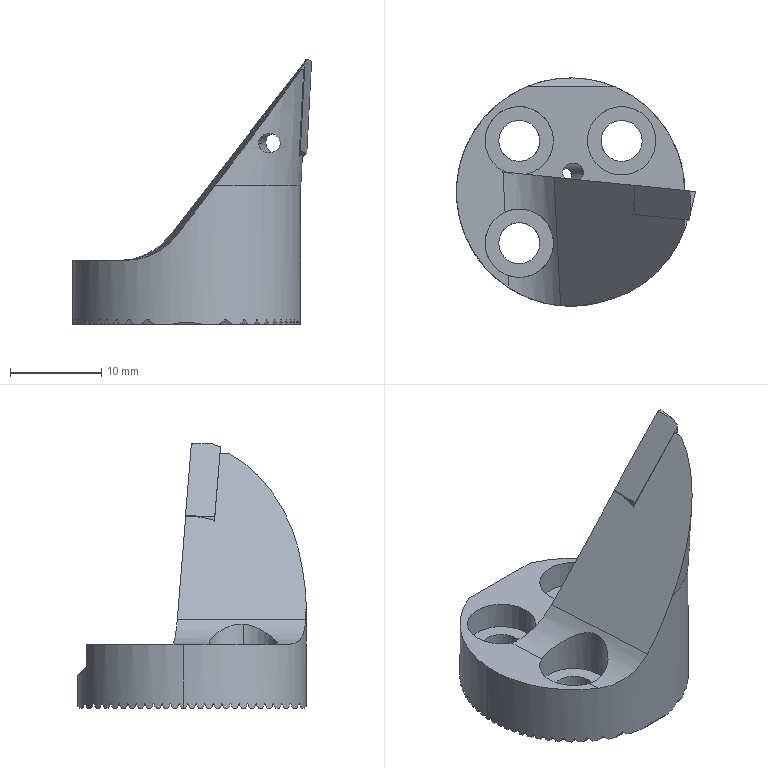CAM job | Mastercam | 3-axis milling, 5-axis milling, drilling
Tools:
tool_number,name,type,diameter_mm,corner_radius_mm,flutes,flute_length_mm,overall_length_mm,shoulder_length_mm,holder_diameter_mm,length_offset,diameter_offset,default_rpm,default_feed_mm_min,default_plunge_mm_min,coolant
1,6 Flat End Mill,end mill,6,0,4,23,23,23,31.877,1,1,1667,200.04,600,COOL_OFF
2,2 Drill,drill,2,0,2,30,30,30,31.877,2,2,3000,360,600,COOL_OFF
4,12 Flat End Mill Rough,end mill,12,0,4,25,25,25,42.012,4,4,833,99.96,600,COOL_OFF
5,3 Flat End Mill Rough,end mill,3,0,4,20,20,20,27.495,5,5,3334,400.08,600,COOL_OFF
6,3 Flat End Mill Rough,end mill,3,0,4,20,20,20,31.877,6,6,3333,399.96,600,COOL_OFF
7,3 Flat End Mill Finish,end mill,3,0,4,20,20,20,31.877,7,7,3333,399.96,600,COOL_OFF
8,2x7deg Chamfer Mill,chamfer mill,6,0,4,12,20,20,31.877,8,8,4167,500.04,600,COOL_OFF
9,12 Flat End Mill Finish,end mill,12,0,4,25,25,25,42.012,9,9,833,99.96,600,COOL_OFF
10,30 Bull Nose Mill,bull end mill,30,0.8,4,30,30,30,50,10,10,400,48,600,COOL_OFF
11,2.5 Flat End Mill,end mill,2.5,0,4,20,20,20,31.877,11,11,4000,480,600,COOL_OFF
12,5 Spot Drill,drill,5,0,2,25,25,25,31.877,12,12,1200,144,600,COOL_OFF
13,2.1 Drill,drill,2.1,0,2,20,20,20,31.877,13,13,2857,342.84,600,COOL_OFF
14,1.95 Thread Mill,thread mill,1.95,0,4,1.35,15,15,31.877,14,14,3077,369.24,600,COOL_OFF
15,2.5 Ball Mill,ball end mill,2.5,1.25,4,3,20,3,31.877,15,15,4800,576,600,COOL_OFF
Operations:
seq,operation,operation_type,tool_number,tool_name,tool_diameter_mm,spindle_rpm,feed_mm_min,plunge_mm_min,retract_mm_min,cycle_time_s,wcs,posted,nc_file
1,2D High Speed (2D Dynamic Mill) - [WCS: Top] - [Tplane: Ins],HighSpeed2D,4,12 Flat End Mill Rough,12,3500,2500,2000,1200,75.295,Top,yes,.nc
2,2D High Speed (2D Dynamic Mill) - [WCS: Top] - [Tplane: Ins-1],HighSpeed2D,4,12 Flat End Mill Rough,12,3500,2500,2000,1200,66.868,Top,yes,.nc
3,Contour (2D) - [WCS: Top] - [Tplane: Out],Contour,1,6 Flat End Mill,6,3500,400,2000,1200,19.183,Top,yes,.nc
4,Peck Drill - [WCS: Top] - [Tplane: Out],Drill,2,2 Drill,2,150,10,600,1200,57.614,Top,yes,.nc
5,2D High Speed (2D Dynamic Mill) - [WCS: Top] - [Tplane: Ins],HighSpeed2D,4,12 Flat End Mill Rough,12,3500,2500,2000,1200,18.885,Top,yes,.nc
6,Contour (2D) - [WCS: Top] - [Tplane: Ins],Contour,4,12 Flat End Mill Rough,12,3500,1000,2000,1200,6.261,Top,yes,.nc
7,Contour (Ramp) - [WCS: Top] - [Tplane: 0d],Contour,4,12 Flat End Mill Rough,12,3500,1500,2000,1200,2.576,Top,yes,.nc
8,Contour (Ramp) - [WCS: Top] - [Tplane: 45d],Contour,4,12 Flat End Mill Rough,12,3500,1500,2000,1200,2.436,Top,yes,.nc
9,Contour (2D) - [WCS: Top] - [Tplane: Ins],Contour,6,3 Flat End Mill Rough,3,4500,400,2000,1200,180.495,Top,yes,.nc
10,Contour (2D) - [WCS: Top] - [Tplane: Ins],Contour,7,3 Flat End Mill Finish,3,4500,400,2000,1200,10.995,Top,yes,.nc
11,Contour (2D) - [WCS: Top] - [Tplane: Ins],Contour,7,3 Flat End Mill Finish,3,4500,400,2000,1200,10.995,Top,yes,.nc
12,Contour (2D chamfer) - [WCS: Top] - [Tplane: Ins],Contour,8,2x7deg Chamfer Mill,6,3500,400,2000,1200,9.64,Top,yes,.nc
13,Contour (2D) - [WCS: Top] - [Tplane: Ins-1],Contour,9,12 Flat End Mill Finish,12,3500,600,2000,1200,5.675,Top,yes,.nc
14,Contour (2D) - [WCS: Top] - [Tplane: Ins],Contour,9,12 Flat End Mill Finish,12,3500,600,2000,1200,4.903,Top,yes,.nc
15,Contour (2D) - [WCS: Top] - [Tplane: 0d],Contour,9,12 Flat End Mill Finish,12,3500,600,2000,1200,3.055,Top,yes,.nc
16,Contour (2D) - [WCS: Top] - [Tplane: 45d],Contour,9,12 Flat End Mill Finish,12,3500,600,2000,1200,2.916,Top,yes,.nc
17,Contour (2D) - [WCS: Top] - [Tplane: Ins],Contour,10,30 Bull Nose Mill,30,3000,400,2000,1200,10.103,Top,yes,.nc
18,Drill/Counterbore - [WCS: Top] - [Tplane: Ins],Drill,12,5 Spot Drill,5,2000,100,600,1200,1.919,Top,yes,.nc
19,Peck Drill - [WCS: Top] - [Tplane: Ins],Drill,13,2.1 Drill,2.1,2500,40,600,1200,14.202,Top,yes,.nc
20,Peck Drill - [WCS: Top] - [Tplane: Plane],Drill,11,2.5 Flat End Mill,2.5,4000,40,600,1200,6.243,Top,yes,.nc
21,Thread Mill - [WCS: Top] - [Tplane: Plane],ThreadMill,14,1.95 Thread Mill,1.95,3000,200,2000,1200,15.959,Top,yes,.nc
22,Deburr 5-axis - [WCS: Top] - [Tplane: Top],459,15,2.5 Ball Mill,2.5,5000,1000,2000,1200,6.126,Top,yes,.nc
23,Deburr 5-axis - [WCS: Top] - [Tplane: Top],459,15,2.5 Ball Mill,2.5,6000,1000,2000,1200,2.974,Top,yes,.nc
24,Stock model - [WCS: Top] - [Tplane: Ins] - 1,139,,,,0,0,0,0,0,Top,yes,.nc